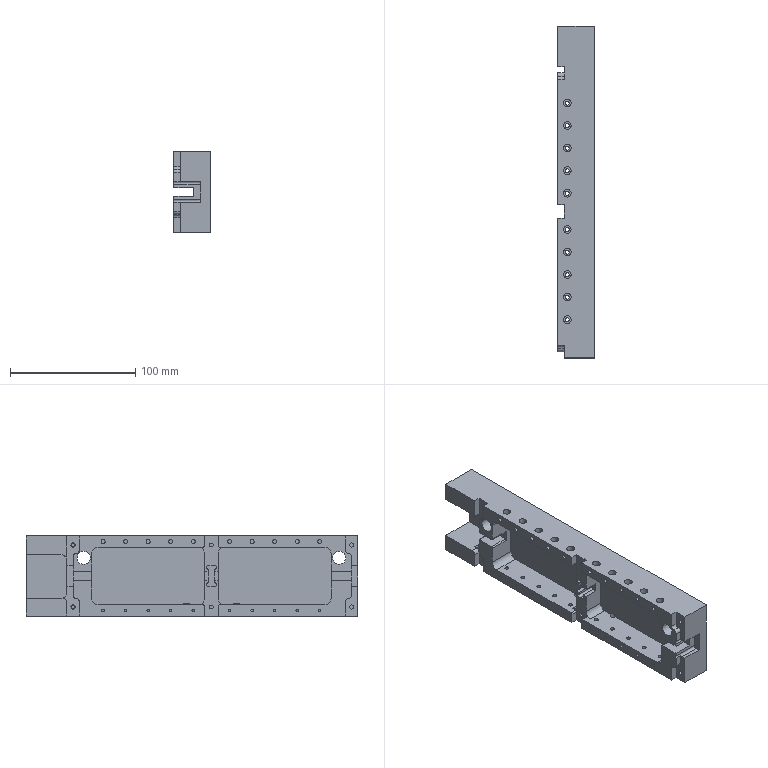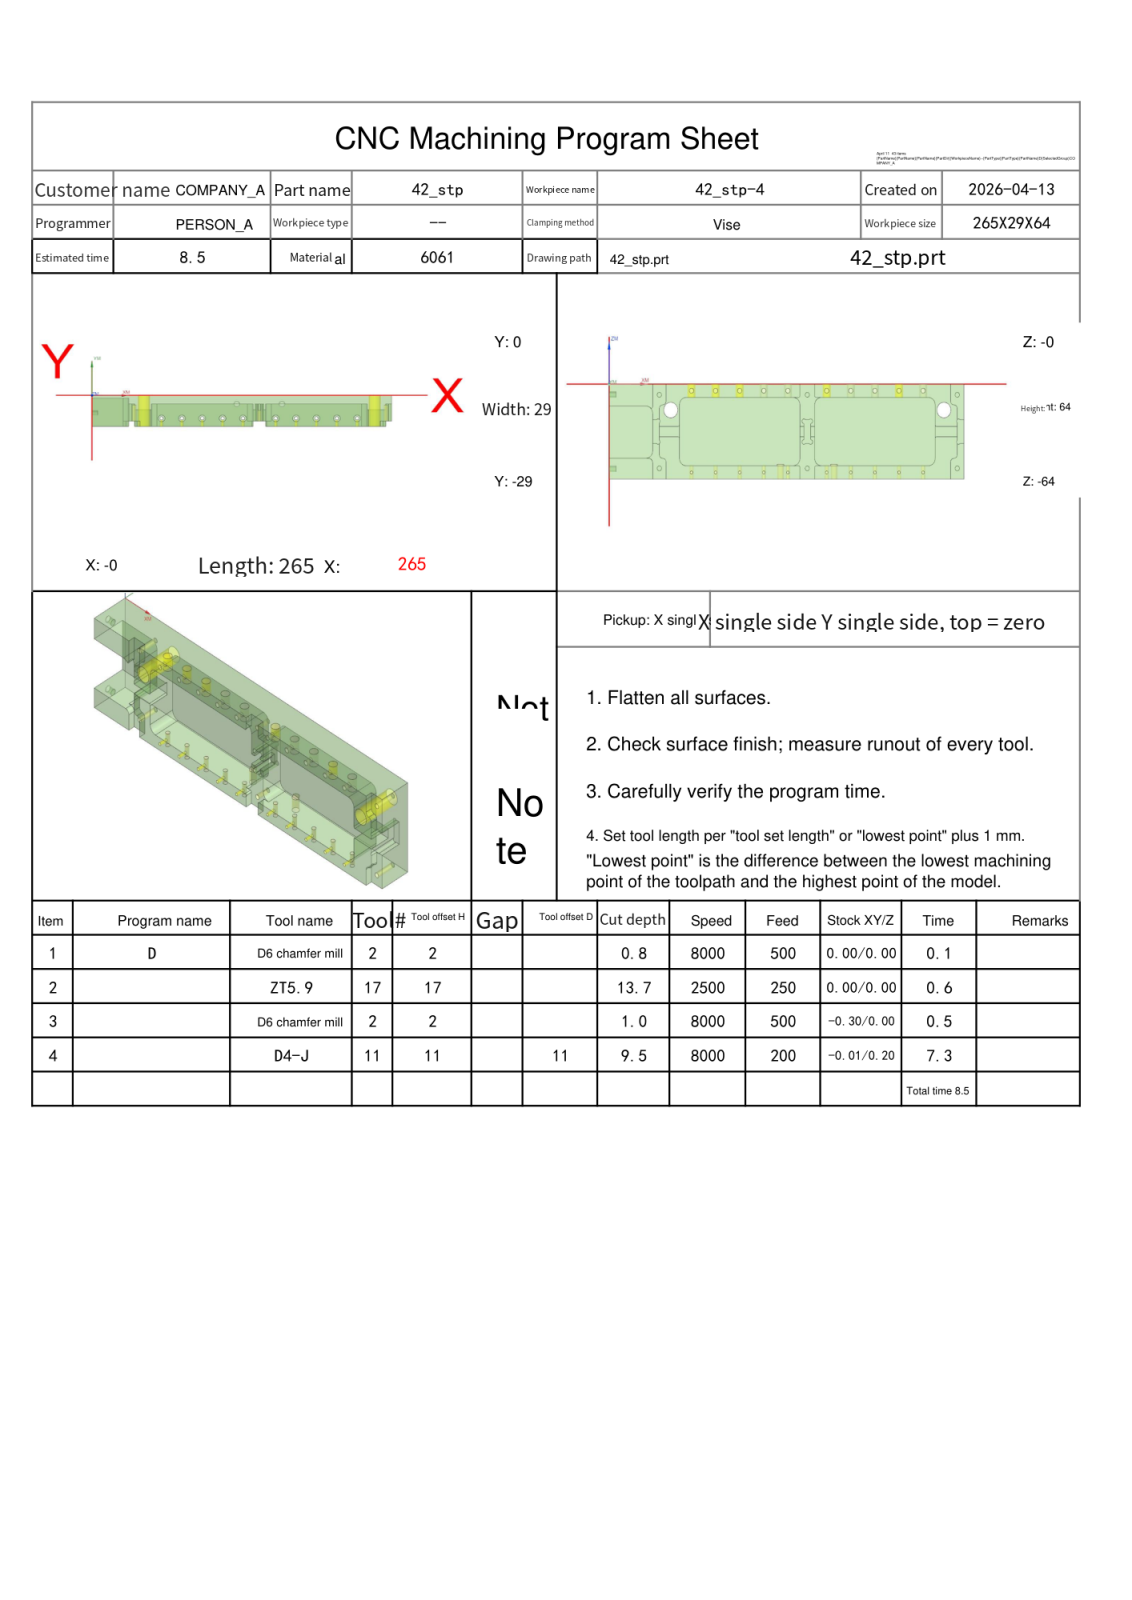NC program | NX | posted by the shop | part box 29 x 265 x 64 mm
Whole program:
%
O0001
(Machine time: 9.17 MIN)
(===Total Tool:3===)
(T2=D6 chamfer mill   D=6.   R=0.   D-  H02 Z=-1.   )
(T17=ZT5.9  D=5.9  DR_a=120 D-  H17 Z=-13.7 )
(T11=D4-J   D=4.   R=0.   D11 H11 Z=-9.5  )
G80 G90 G17 G49 G40
G91 G28 Z0
M01
N1 T02 M06
(D6 chamfer mill  D=6. R=0. H=02 ce=0.00 di=0.00)
G00 G90 G54 X234.5 Y-21.5 M03 S8000
G43 H02 Z20.
M08
G98 G81 X234.5 Y-21.5 Z-.8 R1. F500.
X216.5
X198.5
X180.5
X162.5
X133.5
X115.5
X97.5
X79.5
X61.5
G80
G00 Z20.
G91 G28 Z0.0
M05
M09
G91 G28 Z0.0
M01
N2 T17 M06
(ZT5.9 D=5.9 DR_a=120 H=17)
G00 G90 G54 X234.5 Y-21.5 M03 S2500
G43 H17 Z20.
M08
G98 G83 X234.5 Y-21.5 Z-13.703 R1. F250. Q2.
X216.5
X198.5
X180.5
X162.5
X133.5
X115.5
X97.5
X79.5
X61.5
G80
G00 Z20.
G91 G28 Z0.0
M05
M09
G91 G28 Z0.0
M01
N3 T02 M06
(D6 chamfer mill  D=6. R=0. H=02 ce=-0.30 di=0.00)
G00 G90 G54 X62.675 Y-20.834 M03 S8000
G43 H02 Z20.
M08
Z-.5
G01 Z-1. F500.
X63. Y-20.65
G03 X61.5 Y-19.15 I-1.5 J0.0
X59.15 Y-21.5 I0.0 J-2.35
X61.5 Y-23.85 I2.35 J0.0
X63.85 Y-21.5 I0.0 J2.35
X61.5 Y-19.15 I-2.35 J0.0
X60. Y-20.65 I0.0 J-1.5
G01 X60.325 Y-20.834
Z-.5
G00 Z20.
X80.675
Z-.5
G01 Z-1.
X81. Y-20.65
G03 X79.5 Y-19.15 I-1.5 J0.0
X77.15 Y-21.5 I0.0 J-2.35
X79.5 Y-23.85 I2.35 J0.0
X81.85 Y-21.5 I0.0 J2.35
X79.5 Y-19.15 I-2.35 J0.0
X78. Y-20.65 I0.0 J-1.5
G01 X78.325 Y-20.834
Z-.5
G00 Z20.
X98.675
Z-.5
G01 Z-1.
X99. Y-20.65
G03 X97.5 Y-19.15 I-1.5 J0.0
X95.15 Y-21.5 I0.0 J-2.35
X97.5 Y-23.85 I2.35 J0.0
X99.85 Y-21.5 I0.0 J2.35
X97.5 Y-19.15 I-2.35 J0.0
X96. Y-20.65 I0.0 J-1.5
G01 X96.325 Y-20.834
Z-.5
G00 Z20.
X116.675
Z-.5
G01 Z-1.
X117. Y-20.65
G03 X115.5 Y-19.15 I-1.5 J0.0
X113.15 Y-21.5 I0.0 J-2.35
X115.5 Y-23.85 I2.35 J0.0
X117.85 Y-21.5 I0.0 J2.35
X115.5 Y-19.15 I-2.35 J0.0
X114. Y-20.65 I0.0 J-1.5
G01 X114.325 Y-20.834
Z-.5
G00 Z20.
X132.325 Y-22.166
Z-.5
G01 Z-1.
X132. Y-22.35
G03 X133.5 Y-23.85 I1.5 J0.0
X135.85 Y-21.5 I0.0 J2.35
X133.5 Y-19.15 I-2.35 J0.0
X131.15 Y-21.5 I0.0 J-2.35
X133.5 Y-23.85 I2.35 J0.0
X135. Y-22.35 I0.0 J1.5
G01 X134.675 Y-22.166
Z-.5
G00 Z20.
X161.325
Z-.5
G01 Z-1.
X161. Y-22.35
G03 X162.5 Y-23.85 I1.5 J0.0
X164.85 Y-21.5 I0.0 J2.35
X162.5 Y-19.15 I-2.35 J0.0
X160.15 Y-21.5 I0.0 J-2.35
X162.5 Y-23.85 I2.35 J0.0
X164. Y-22.35 I0.0 J1.5
G01 X163.675 Y-22.166
Z-.5
G00 Z20.
X181.675 Y-20.834
Z-.5
G01 Z-1.
X182. Y-20.65
G03 X180.5 Y-19.15 I-1.5 J0.0
X178.15 Y-21.5 I0.0 J-2.35
X180.5 Y-23.85 I2.35 J0.0
X182.85 Y-21.5 I0.0 J2.35
X180.5 Y-19.15 I-2.35 J0.0
X179. Y-20.65 I0.0 J-1.5
G01 X179.325 Y-20.834
Z-.5
G00 Z20.
X199.675
Z-.5
G01 Z-1.
X200. Y-20.65
G03 X198.5 Y-19.15 I-1.5 J0.0
X196.15 Y-21.5 I0.0 J-2.35
X198.5 Y-23.85 I2.35 J0.0
X200.85 Y-21.5 I0.0 J2.35
X198.5 Y-19.15 I-2.35 J0.0
X197. Y-20.65 I0.0 J-1.5
G01 X197.325 Y-20.834
Z-.5
G00 Z20.
X217.675
Z-.5
G01 Z-1.
X218. Y-20.65
G03 X216.5 Y-19.15 I-1.5 J0.0
X214.15 Y-21.5 I0.0 J-2.35
X216.5 Y-23.85 I2.35 J0.0
X218.85 Y-21.5 I0.0 J2.35
X216.5 Y-19.15 I-2.35 J0.0
X215. Y-20.65 I0.0 J-1.5
G01 X215.325 Y-20.834
Z-.5
G00 Z20.
X235.675
Z-.5
G01 Z-1.
X236. Y-20.65
G03 X234.5 Y-19.15 I-1.5 J0.0
X232.15 Y-21.5 I0.0 J-2.35
X234.5 Y-23.85 I2.35 J0.0
X236.85 Y-21.5 I0.0 J2.35
X234.5 Y-19.15 I-2.35 J0.0
X233. Y-20.65 I0.0 J-1.5
G01 X233.325 Y-20.834
Z-.5
G00 Z20.
G91 G28 Z0.0
M05
M09
G91 G28 Z0.0
M01
N4 T11 M06
(D4-J  D=4. R=0. H=11 ce=-0.01 di=0.20)
G00 G90 G54 X97.5 Y-21.5 M03 S8000
G43 H11 Z20.
M08
Z.5
G41 D11
G01 X97.686 Y-21.427 F200.
G03 X98.011 Y-20.951 I-.186 J.476
X97.5 Y-20.44 I-.511 J0.0
X97.5 Y-20.44 Z0.0 I0.0 J-1.06
X97.5 Y-20.44 Z-.5 I0.0 J-1.06
X97.5 Y-20.44 Z-1. I0.0 J-1.06
X97.5 Y-20.44 Z-1.5 I0.0 J-1.06
X97.5 Y-20.44 Z-2. I0.0 J-1.06
X97.5 Y-20.44 Z-2.5 I0.0 J-1.06
X97.5 Y-20.44 Z-3. I0.0 J-1.06
X97.5 Y-20.44 Z-3.5 I0.0 J-1.06
X97.5 Y-20.44 Z-4. I0.0 J-1.06
X97.5 Y-20.44 Z-4.5 I0.0 J-1.06
X97.5 Y-20.44 Z-5. I0.0 J-1.06
X97.5 Y-20.44 Z-5.5 I0.0 J-1.06
X97.5 Y-20.44 Z-6. I0.0 J-1.06
X97.5 Y-20.44 Z-6.5 I0.0 J-1.06
X97.5 Y-20.44 Z-7. I0.0 J-1.06
X97.5 Y-20.44 Z-7.5 I0.0 J-1.06
X97.5 Y-20.44 Z-8. I0.0 J-1.06
X97.5 Y-20.44 Z-8.5 I0.0 J-1.06
X97.5 Y-20.44 Z-9. I0.0 J-1.06
X97.5 Y-20.44 Z-9.5 I0.0 J-1.06
X96.44 Y-21.5 I0.0 J-1.06
X97.5 Y-22.56 I1.06 J0.0
X98.56 Y-21.5 I0.0 J1.06
X97.5 Y-20.44 I-1.06 J0.0
X96.989 Y-20.951 I0.0 J-.511
X97.314 Y-21.427 I.511 J0.0
G01 G40 X97.5 Y-21.5
G00 Z20.
X79.5
Z.5
G41 D11
G01 X79.686 Y-21.427
G03 X80.011 Y-20.951 I-.186 J.476
X79.5 Y-20.44 I-.511 J0.0
X79.5 Y-20.44 Z0.0 I0.0 J-1.06
X79.5 Y-20.44 Z-.5 I0.0 J-1.06
X79.5 Y-20.44 Z-1. I0.0 J-1.06
X79.5 Y-20.44 Z-1.5 I0.0 J-1.06
X79.5 Y-20.44 Z-2. I0.0 J-1.06
X79.5 Y-20.44 Z-2.5 I0.0 J-1.06
X79.5 Y-20.44 Z-3. I0.0 J-1.06
X79.5 Y-20.44 Z-3.5 I0.0 J-1.06
X79.5 Y-20.44 Z-4. I0.0 J-1.06
X79.5 Y-20.44 Z-4.5 I0.0 J-1.06
X79.5 Y-20.44 Z-5. I0.0 J-1.06
X79.5 Y-20.44 Z-5.5 I0.0 J-1.06
X79.5 Y-20.44 Z-6. I0.0 J-1.06
X79.5 Y-20.44 Z-6.5 I0.0 J-1.06
X79.5 Y-20.44 Z-7. I0.0 J-1.06
X79.5 Y-20.44 Z-7.5 I0.0 J-1.06
X79.5 Y-20.44 Z-8. I0.0 J-1.06
X79.5 Y-20.44 Z-8.5 I0.0 J-1.06
X79.5 Y-20.44 Z-9. I0.0 J-1.06
X79.5 Y-20.44 Z-9.5 I0.0 J-1.06
X78.44 Y-21.5 I0.0 J-1.06
X79.5 Y-22.56 I1.06 J0.0
X80.56 Y-21.5 I0.0 J1.06
X79.5 Y-20.44 I-1.06 J0.0
X78.989 Y-20.951 I0.0 J-.511
X79.314 Y-21.427 I.511 J0.0
G01 G40 X79.5 Y-21.5
G00 Z20.
X61.5
Z.5
G41 D11
G01 X61.686 Y-21.427
G03 X62.011 Y-20.951 I-.186 J.476
X61.5 Y-20.44 I-.511 J0.0
X61.5 Y-20.44 Z0.0 I0.0 J-1.06
X61.5 Y-20.44 Z-.5 I0.0 J-1.06
X61.5 Y-20.44 Z-1. I0.0 J-1.06
X61.5 Y-20.44 Z-1.5 I0.0 J-1.06
X61.5 Y-20.44 Z-2. I0.0 J-1.06
X61.5 Y-20.44 Z-2.5 I0.0 J-1.06
X61.5 Y-20.44 Z-3. I0.0 J-1.06
X61.5 Y-20.44 Z-3.5 I0.0 J-1.06
X61.5 Y-20.44 Z-4. I0.0 J-1.06
X61.5 Y-20.44 Z-4.5 I0.0 J-1.06
X61.5 Y-20.44 Z-5. I0.0 J-1.06
X61.5 Y-20.44 Z-5.5 I0.0 J-1.06
X61.5 Y-20.44 Z-6. I0.0 J-1.06
X61.5 Y-20.44 Z-6.5 I0.0 J-1.06
X61.5 Y-20.44 Z-7. I0.0 J-1.06
X61.5 Y-20.44 Z-7.5 I0.0 J-1.06
X61.5 Y-20.44 Z-8. I0.0 J-1.06
X61.5 Y-20.44 Z-8.5 I0.0 J-1.06
X61.5 Y-20.44 Z-9. I0.0 J-1.06
X61.5 Y-20.44 Z-9.5 I0.0 J-1.06
X60.44 Y-21.5 I0.0 J-1.06
X61.5 Y-22.56 I1.06 J0.0
X62.56 Y-21.5 I0.0 J1.06
X61.5 Y-20.44 I-1.06 J0.0
X60.989 Y-20.951 I0.0 J-.511
X61.314 Y-21.427 I.511 J0.0
G01 G40 X61.5 Y-21.5
G00 Z20.
X162.5
Z.5
G41 D11
G01 X162.686 Y-21.427
G03 X163.011 Y-20.951 I-.186 J.476
X162.5 Y-20.44 I-.511 J0.0
X162.5 Y-20.44 Z0.0 I0.0 J-1.06
X162.5 Y-20.44 Z-.5 I0.0 J-1.06
X162.5 Y-20.44 Z-1. I0.0 J-1.06
X162.5 Y-20.44 Z-1.5 I0.0 J-1.06
X162.5 Y-20.44 Z-2. I0.0 J-1.06
X162.5 Y-20.44 Z-2.5 I0.0 J-1.06
X162.5 Y-20.44 Z-3. I0.0 J-1.06
X162.5 Y-20.44 Z-3.5 I0.0 J-1.06
X162.5 Y-20.44 Z-4. I0.0 J-1.06
X162.5 Y-20.44 Z-4.5 I0.0 J-1.06
X162.5 Y-20.44 Z-5. I0.0 J-1.06
X162.5 Y-20.44 Z-5.5 I0.0 J-1.06
X162.5 Y-20.44 Z-6. I0.0 J-1.06
X162.5 Y-20.44 Z-6.5 I0.0 J-1.06
X162.5 Y-20.44 Z-7. I0.0 J-1.06
X162.5 Y-20.44 Z-7.5 I0.0 J-1.06
X162.5 Y-20.44 Z-8. I0.0 J-1.06
X162.5 Y-20.44 Z-8.5 I0.0 J-1.06
X162.5 Y-20.44 Z-9. I0.0 J-1.06
X162.5 Y-20.44 Z-9.5 I0.0 J-1.06
X161.44 Y-21.5 I0.0 J-1.06
X162.5 Y-22.56 I1.06 J0.0
X163.56 Y-21.5 I0.0 J1.06
X162.5 Y-20.44 I-1.06 J0.0
X161.989 Y-20.951 I0.0 J-.511
X162.314 Y-21.427 I.511 J0.0
G01 G40 X162.5 Y-21.5
G00 Z20.
X216.5
Z.5
G41 D11
G01 X216.686 Y-21.427
G03 X217.011 Y-20.951 I-.186 J.476
X216.5 Y-20.44 I-.511 J0.0
X216.5 Y-20.44 Z0.0 I0.0 J-1.06
X216.5 Y-20.44 Z-.5 I0.0 J-1.06
X216.5 Y-20.44 Z-1. I0.0 J-1.06
X216.5 Y-20.44 Z-1.5 I0.0 J-1.06
X216.5 Y-20.44 Z-2. I0.0 J-1.06
X216.5 Y-20.44 Z-2.5 I0.0 J-1.06
X216.5 Y-20.44 Z-3. I0.0 J-1.06
X216.5 Y-20.44 Z-3.5 I0.0 J-1.06
X216.5 Y-20.44 Z-4. I0.0 J-1.06
X216.5 Y-20.44 Z-4.5 I0.0 J-1.06
X216.5 Y-20.44 Z-5. I0.0 J-1.06
X216.5 Y-20.44 Z-5.5 I0.0 J-1.06
X216.5 Y-20.44 Z-6. I0.0 J-1.06
X216.5 Y-20.44 Z-6.5 I0.0 J-1.06
X216.5 Y-20.44 Z-7. I0.0 J-1.06
X216.5 Y-20.44 Z-7.5 I0.0 J-1.06
X216.5 Y-20.44 Z-8. I0.0 J-1.06
X216.5 Y-20.44 Z-8.5 I0.0 J-1.06
X216.5 Y-20.44 Z-9. I0.0 J-1.06
X216.5 Y-20.44 Z-9.5 I0.0 J-1.06
X215.44 Y-21.5 I0.0 J-1.06
X216.5 Y-22.56 I1.06 J0.0
X217.56 Y-21.5 I0.0 J1.06
X216.5 Y-20.44 I-1.06 J0.0
X215.989 Y-20.951 I0.0 J-.511
X216.314 Y-21.427 I.511 J0.0
G01 G40 X216.5 Y-21.5
G00 Z20.
G00 G90 X198.5 Y-21.5 M03 S8000
Z20.
Z.5
G41 D11
G01 X198.686 Y-21.427 F200.
G03 X199.011 Y-20.951 I-.186 J.476
X198.5 Y-20.44 I-.511 J0.0
X198.5 Y-20.44 Z0.0 I0.0 J-1.06
X198.5 Y-20.44 Z-.5 I0.0 J-1.06
X198.5 Y-20.44 Z-1. I0.0 J-1.06
X198.5 Y-20.44 Z-1.5 I0.0 J-1.06
X198.5 Y-20.44 Z-2. I0.0 J-1.06
X198.5 Y-20.44 Z-2.5 I0.0 J-1.06
X198.5 Y-20.44 Z-3. I0.0 J-1.06
X198.5 Y-20.44 Z-3.5 I0.0 J-1.06
X198.5 Y-20.44 Z-4. I0.0 J-1.06
X198.5 Y-20.44 Z-4.5 I0.0 J-1.06
X198.5 Y-20.44 Z-5. I0.0 J-1.06
X198.5 Y-20.44 Z-5.5 I0.0 J-1.06
X198.5 Y-20.44 Z-6. I0.0 J-1.06
X198.5 Y-20.44 Z-6.5 I0.0 J-1.06
X198.5 Y-20.44 Z-7. I0.0 J-1.06
X198.5 Y-20.44 Z-7.5 I0.0 J-1.06
X198.5 Y-20.44 Z-8. I0.0 J-1.06
X198.5 Y-20.44 Z-8.5 I0.0 J-1.06
X198.5 Y-20.44 Z-9. I0.0 J-1.06
X198.5 Y-20.44 Z-9.5 I0.0 J-1.06
X197.44 Y-21.5 I0.0 J-1.06
X198.5 Y-22.56 I1.06 J0.0
X199.56 Y-21.5 I0.0 J1.06
X198.5 Y-20.44 I-1.06 J0.0
X197.989 Y-20.951 I0.0 J-.511
X198.314 Y-21.427 I.511 J0.0
G01 G40 X198.5 Y-21.5
G00 Z20.
X234.5
Z.5
G41 D11
G01 X234.686 Y-21.427
G03 X235.011 Y-20.951 I-.186 J.476
X234.5 Y-20.44 I-.511 J0.0
X234.5 Y-20.44 Z0.0 I0.0 J-1.06
X234.5 Y-20.44 Z-.5 I0.0 J-1.06
X234.5 Y-20.44 Z-1. I0.0 J-1.06
X234.5 Y-20.44 Z-1.5 I0.0 J-1.06
X234.5 Y-20.44 Z-2. I0.0 J-1.06
X234.5 Y-20.44 Z-2.5 I0.0 J-1.06
X234.5 Y-20.44 Z-3. I0.0 J-1.06
X234.5 Y-20.44 Z-3.5 I0.0 J-1.06
X234.5 Y-20.44 Z-4. I0.0 J-1.06
X234.5 Y-20.44 Z-4.5 I0.0 J-1.06
X234.5 Y-20.44 Z-5. I0.0 J-1.06
X234.5 Y-20.44 Z-5.5 I0.0 J-1.06
X234.5 Y-20.44 Z-6. I0.0 J-1.06
X234.5 Y-20.44 Z-6.5 I0.0 J-1.06
X234.5 Y-20.44 Z-7. I0.0 J-1.06
X234.5 Y-20.44 Z-7.5 I0.0 J-1.06
X234.5 Y-20.44 Z-8. I0.0 J-1.06
X234.5 Y-20.44 Z-8.5 I0.0 J-1.06
X234.5 Y-20.44 Z-9. I0.0 J-1.06
X234.5 Y-20.44 Z-9.5 I0.0 J-1.06
X233.44 Y-21.5 I0.0 J-1.06
X234.5 Y-22.56 I1.06 J0.0
X235.56 Y-21.5 I0.0 J1.06
X234.5 Y-20.44 I-1.06 J0.0
X233.989 Y-20.951 I0.0 J-.511
X234.314 Y-21.427 I.511 J0.0
G01 G40 X234.5 Y-21.5
G00 Z20.
X180.5
Z.5
G41 D11
G01 X180.686 Y-21.427
G03 X181.011 Y-20.951 I-.186 J.476
X180.5 Y-20.44 I-.511 J0.0
X180.5 Y-20.44 Z0.0 I0.0 J-1.06
X180.5 Y-20.44 Z-.5 I0.0 J-1.06
X180.5 Y-20.44 Z-1. I0.0 J-1.06
X180.5 Y-20.44 Z-1.5 I0.0 J-1.06
X180.5 Y-20.44 Z-2. I0.0 J-1.06
X180.5 Y-20.44 Z-2.5 I0.0 J-1.06
X180.5 Y-20.44 Z-3. I0.0 J-1.06
X180.5 Y-20.44 Z-3.5 I0.0 J-1.06
X180.5 Y-20.44 Z-4. I0.0 J-1.06
X180.5 Y-20.44 Z-4.5 I0.0 J-1.06
X180.5 Y-20.44 Z-5. I0.0 J-1.06
X180.5 Y-20.44 Z-5.5 I0.0 J-1.06
X180.5 Y-20.44 Z-6. I0.0 J-1.06
X180.5 Y-20.44 Z-6.5 I0.0 J-1.06
X180.5 Y-20.44 Z-7. I0.0 J-1.06
X180.5 Y-20.44 Z-7.5 I0.0 J-1.06
X180.5 Y-20.44 Z-8. I0.0 J-1.06
X180.5 Y-20.44 Z-8.5 I0.0 J-1.06
X180.5 Y-20.44 Z-9. I0.0 J-1.06
X180.5 Y-20.44 Z-9.5 I0.0 J-1.06
X179.44 Y-21.5 I0.0 J-1.06
X180.5 Y-22.56 I1.06 J0.0
X181.56 Y-21.5 I0.0 J1.06
X180.5 Y-20.44 I-1.06 J0.0
X179.989 Y-20.951 I0.0 J-.511
X180.314 Y-21.427 I.511 J0.0
G01 G40 X180.5 Y-21.5
G00 Z20.
X133.5
Z.5
G41 D11
G01 X133.686 Y-21.427
G03 X134.011 Y-20.951 I-.186 J.476
X133.5 Y-20.44 I-.511 J0.0
X133.5 Y-20.44 Z0.0 I0.0 J-1.06
X133.5 Y-20.44 Z-.5 I0.0 J-1.06
X133.5 Y-20.44 Z-1. I0.0 J-1.06
X133.5 Y-20.44 Z-1.5 I0.0 J-1.06
X133.5 Y-20.44 Z-2. I0.0 J-1.06
X133.5 Y-20.44 Z-2.5 I0.0 J-1.06
X133.5 Y-20.44 Z-3. I0.0 J-1.06
X133.5 Y-20.44 Z-3.5 I0.0 J-1.06
X133.5 Y-20.44 Z-4. I0.0 J-1.06
X133.5 Y-20.44 Z-4.5 I0.0 J-1.06
X133.5 Y-20.44 Z-5. I0.0 J-1.06
X133.5 Y-20.44 Z-5.5 I0.0 J-1.06
X133.5 Y-20.44 Z-6. I0.0 J-1.06
X133.5 Y-20.44 Z-6.5 I0.0 J-1.06
X133.5 Y-20.44 Z-7. I0.0 J-1.06
X133.5 Y-20.44 Z-7.5 I0.0 J-1.06
X133.5 Y-20.44 Z-8. I0.0 J-1.06
X133.5 Y-20.44 Z-8.5 I0.0 J-1.06
X133.5 Y-20.44 Z-9. I0.0 J-1.06
X133.5 Y-20.44 Z-9.5 I0.0 J-1.06
X132.44 Y-21.5 I0.0 J-1.06
X133.5 Y-22.56 I1.06 J0.0
X134.56 Y-21.5 I0.0 J1.06
X133.5 Y-20.44 I-1.06 J0.0
X132.989 Y-20.951 I0.0 J-.511
X133.314 Y-21.427 I.511 J0.0
G01 G40 X133.5 Y-21.5
G00 Z20.
X115.5
Z.5
G41 D11
G01 X115.686 Y-21.427
G03 X116.011 Y-20.951 I-.186 J.476
X115.5 Y-20.44 I-.511 J0.0
X115.5 Y-20.44 Z0.0 I0.0 J-1.06
X115.5 Y-20.44 Z-.5 I0.0 J-1.06
X115.5 Y-20.44 Z-1. I0.0 J-1.06
X115.5 Y-20.44 Z-1.5 I0.0 J-1.06
X115.5 Y-20.44 Z-2. I0.0 J-1.06
X115.5 Y-20.44 Z-2.5 I0.0 J-1.06
X115.5 Y-20.44 Z-3. I0.0 J-1.06
X115.5 Y-20.44 Z-3.5 I0.0 J-1.06
X115.5 Y-20.44 Z-4. I0.0 J-1.06
X115.5 Y-20.44 Z-4.5 I0.0 J-1.06
X115.5 Y-20.44 Z-5. I0.0 J-1.06
X115.5 Y-20.44 Z-5.5 I0.0 J-1.06
X115.5 Y-20.44 Z-6. I0.0 J-1.06
X115.5 Y-20.44 Z-6.5 I0.0 J-1.06
X115.5 Y-20.44 Z-7. I0.0 J-1.06
X115.5 Y-20.44 Z-7.5 I0.0 J-1.06
X115.5 Y-20.44 Z-8. I0.0 J-1.06
X115.5 Y-20.44 Z-8.5 I0.0 J-1.06
X115.5 Y-20.44 Z-9. I0.0 J-1.06
X115.5 Y-20.44 Z-9.5 I0.0 J-1.06
X114.44 Y-21.5 I0.0 J-1.06
X115.5 Y-22.56 I1.06 J0.0
X116.56 Y-21.5 I0.0 J1.06
X115.5 Y-20.44 I-1.06 J0.0
X114.989 Y-20.951 I0.0 J-.511
X115.314 Y-21.427 I.511 J0.0
G01 G40 X115.5 Y-21.5
G00 Z20.
M05
M09
G91 G28 Z0.0
G91 G28 Y0.0
M30
%